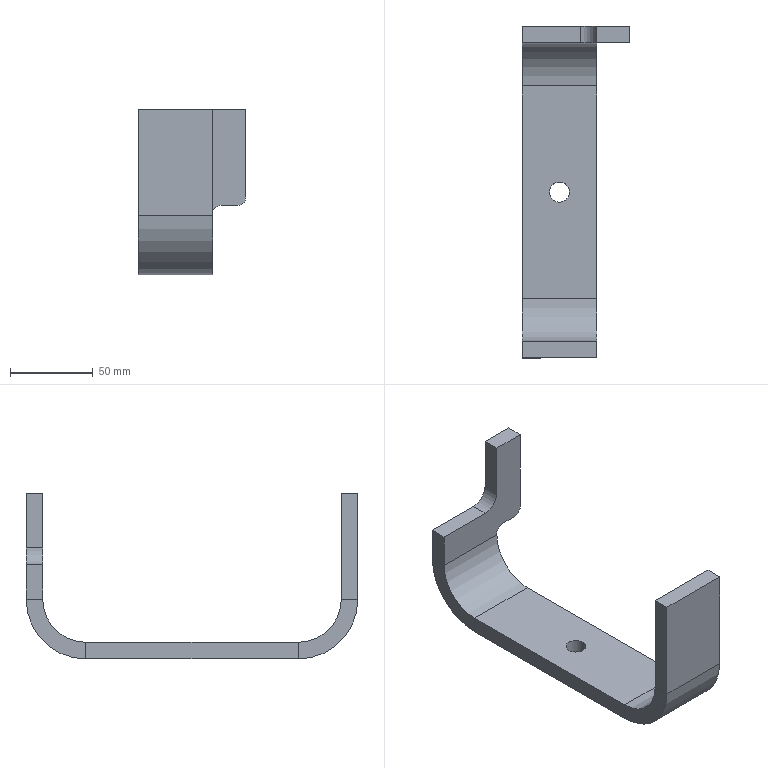Part | SolidWorks | features Cut 1, FlatPattern 1, SM3dBend 1, SMBaseFlange 1, SheetMetal 1 | 1 solid | 31 faces | box 65 x 200.003 x 99.994 mm | volume 150355 mm3 | plane 22 | cylinder 9 | commonest cylinder face diameters 10 x2 12 x2 52 x2 72 x2 20 x1
STEP:
#1=CARTESIAN_POINT('',(-38.456,6.751,0.));
#2=VERTEX_POINT('',#1);
#3=CARTESIAN_POINT('',(-26.456,6.751,0.));
#4=VERTEX_POINT('',#3);
#5=CARTESIAN_POINT('',(-32.456,6.751,0.));
#6=DIRECTION('',(0.,0.,1.));
#7=DIRECTION('',(1.,0.,0.));
#8=AXIS2_PLACEMENT_3D('',#5,#6,#7);
#9=CIRCLE('',#8,6.);
#10=EDGE_CURVE('',#2,#4,#9,.T.);
#11=ORIENTED_EDGE('',*,*,#10,.T.);
#12=CARTESIAN_POINT('',(-26.456,6.751,-10.));
#13=VERTEX_POINT('',#12);
#14=CARTESIAN_POINT('',(-26.456,6.751,89.994));
#15=DIRECTION('',(0.,0.,-1.));
#16=VECTOR('',#15,1000.);
#17=LINE('',#14,#16);
#18=EDGE_CURVE('',#4,#13,#17,.T.);
#19=ORIENTED_EDGE('',*,*,#18,.T.);
#20=CARTESIAN_POINT('',(-38.456,6.751,-10.));
#21=VERTEX_POINT('',#20);
#22=CARTESIAN_POINT('',(-32.456,6.751,-10.));
#23=DIRECTION('',(0.,0.,-1.));
#24=DIRECTION('',(-1.,0.,0.));
#25=AXIS2_PLACEMENT_3D('',#22,#23,#24);
#26=CIRCLE('',#25,6.);
#27=EDGE_CURVE('',#13,#21,#26,.T.);
#28=ORIENTED_EDGE('',*,*,#27,.T.);
#29=CARTESIAN_POINT('',(-38.456,6.751,89.994));
#30=DIRECTION('',(0.,0.,-1.));
#31=VECTOR('',#30,1000.);
#32=LINE('',#29,#31);
#33=EDGE_CURVE('',#2,#21,#32,.T.);
#34=ORIENTED_EDGE('',*,*,#33,.F.);
#35=EDGE_LOOP('',(#11,#19,#28,#34));
#36=FACE_OUTER_BOUND('',#35,.T.);
#37=CARTESIAN_POINT('',(-32.456,6.751,89.994));
#38=DIRECTION('',(0.,0.,-1.));
#39=DIRECTION('',(-1.,0.,0.));
#40=AXIS2_PLACEMENT_3D('',#37,#38,#39);
#41=CYLINDRICAL_SURFACE('',#40,6.);
#42=ADVANCED_FACE('',(#36),#41,.F.);
#43=CARTESIAN_POINT('',(-54.956,70.753,-10.));
#44=VERTEX_POINT('',#43);
#45=CARTESIAN_POINT('',(-54.956,-57.25,-10.));
#46=VERTEX_POINT('',#45);
#47=CARTESIAN_POINT('',(-54.956,-169.939,-10.));
#48=DIRECTION('',(0.,-1.,0.));
#49=VECTOR('',#48,1000.);
#50=LINE('',#47,#49);
#51=EDGE_CURVE('',#44,#46,#50,.T.);
#52=ORIENTED_EDGE('',*,*,#51,.T.);
#53=CARTESIAN_POINT('',(-54.956,-57.25,0.));
#54=VERTEX_POINT('',#53);
#55=CARTESIAN_POINT('',(-54.956,-57.25,-10.));
#56=DIRECTION('',(0.,0.,1.));
#57=VECTOR('',#56,1000.);
#58=LINE('',#55,#57);
#59=EDGE_CURVE('',#46,#54,#58,.T.);
#60=ORIENTED_EDGE('',*,*,#59,.T.);
#61=CARTESIAN_POINT('',(-54.956,70.753,0.));
#62=VERTEX_POINT('',#61);
#63=CARTESIAN_POINT('',(-54.956,-169.939,0.));
#64=DIRECTION('',(0.,-1.,0.));
#65=VECTOR('',#64,1000.);
#66=LINE('',#63,#65);
#67=EDGE_CURVE('',#62,#54,#66,.T.);
#68=ORIENTED_EDGE('',*,*,#67,.F.);
#69=CARTESIAN_POINT('',(-54.956,70.753,-10.));
#70=DIRECTION('',(0.,0.,1.));
#71=VECTOR('',#70,1000.);
#72=LINE('',#69,#71);
#73=EDGE_CURVE('',#44,#62,#72,.T.);
#74=ORIENTED_EDGE('',*,*,#73,.F.);
#75=EDGE_LOOP('',(#52,#60,#68,#74));
#76=FACE_OUTER_BOUND('',#75,.T.);
#77=CARTESIAN_POINT('',(-54.956,-169.939,-10.));
#78=DIRECTION('',(-1.,0.,0.));
#79=DIRECTION('',(0.,-1.,0.));
#80=AXIS2_PLACEMENT_3D('',#77,#78,#79);
#81=PLANE('',#80);
#82=ADVANCED_FACE('',(#76),#81,.T.);
#83=CARTESIAN_POINT('',(-9.956,-57.25,0.));
#84=VERTEX_POINT('',#83);
#85=CARTESIAN_POINT('',(-9.956,70.753,0.));
#86=VERTEX_POINT('',#85);
#87=CARTESIAN_POINT('',(-9.956,120.441,0.));
#88=DIRECTION('',(0.,1.,0.));
#89=VECTOR('',#88,1000.);
#90=LINE('',#87,#89);
#91=EDGE_CURVE('',#84,#86,#90,.T.);
#92=ORIENTED_EDGE('',*,*,#91,.F.);
#93=CARTESIAN_POINT('',(-9.956,-57.25,-10.));
#94=VERTEX_POINT('',#93);
#95=CARTESIAN_POINT('',(-9.956,-57.25,-10.));
#96=DIRECTION('',(0.,0.,-1.));
#97=VECTOR('',#96,1000.);
#98=LINE('',#95,#97);
#99=EDGE_CURVE('',#84,#94,#98,.T.);
#100=ORIENTED_EDGE('',*,*,#99,.T.);
#101=CARTESIAN_POINT('',(-9.956,70.753,-10.));
#102=VERTEX_POINT('',#101);
#103=CARTESIAN_POINT('',(-9.956,120.441,-10.));
#104=DIRECTION('',(0.,1.,0.));
#105=VECTOR('',#104,1000.);
#106=LINE('',#103,#105);
#107=EDGE_CURVE('',#94,#102,#106,.T.);
#108=ORIENTED_EDGE('',*,*,#107,.T.);
#109=CARTESIAN_POINT('',(-9.956,70.753,-10.));
#110=DIRECTION('',(0.,0.,-1.));
#111=VECTOR('',#110,1000.);
#112=LINE('',#109,#111);
#113=EDGE_CURVE('',#86,#102,#112,.T.);
#114=ORIENTED_EDGE('',*,*,#113,.F.);
#115=EDGE_LOOP('',(#92,#100,#108,#114));
#116=FACE_OUTER_BOUND('',#115,.T.);
#117=CARTESIAN_POINT('',(-9.956,120.441,-10.));
#118=DIRECTION('',(1.,0.,0.));
#119=DIRECTION('',(0.,0.,-1.));
#120=AXIS2_PLACEMENT_3D('',#117,#118,#119);
#121=PLANE('',#120);
#122=ADVANCED_FACE('',(#116),#121,.T.);
#123=ORIENTED_EDGE('',*,*,#10,.F.);
#124=CARTESIAN_POINT('',(-32.456,6.751,0.));
#125=DIRECTION('',(0.,0.,1.));
#126=DIRECTION('',(1.,0.,0.));
#127=AXIS2_PLACEMENT_3D('',#124,#125,#126);
#128=CIRCLE('',#127,6.);
#129=EDGE_CURVE('',#4,#2,#128,.T.);
#130=ORIENTED_EDGE('',*,*,#129,.F.);
#131=EDGE_LOOP('',(#123,#130));
#132=FACE_BOUND('',#131,.T.);
#133=ORIENTED_EDGE('',*,*,#67,.T.);
#134=CARTESIAN_POINT('',(-19.956,-57.25,0.));
#135=DIRECTION('',(1.,0.,0.));
#136=VECTOR('',#135,1000.);
#137=LINE('',#134,#136);
#138=EDGE_CURVE('',#54,#84,#137,.T.);
#139=ORIENTED_EDGE('',*,*,#138,.T.);
#140=ORIENTED_EDGE('',*,*,#91,.T.);
#141=CARTESIAN_POINT('',(-19.956,70.753,0.));
#142=DIRECTION('',(1.,0.,0.));
#143=VECTOR('',#142,1000.);
#144=LINE('',#141,#143);
#145=EDGE_CURVE('',#62,#86,#144,.T.);
#146=ORIENTED_EDGE('',*,*,#145,.F.);
#147=EDGE_LOOP('',(#133,#139,#140,#146));
#148=FACE_OUTER_BOUND('',#147,.T.);
#149=CARTESIAN_POINT('',(-19.956,150.441,0.));
#150=DIRECTION('',(0.,0.,1.));
#151=DIRECTION('',(1.,0.,0.));
#152=AXIS2_PLACEMENT_3D('',#149,#150,#151);
#153=PLANE('',#152);
#154=ADVANCED_FACE('',(#132,#148),#153,.T.);
#155=CARTESIAN_POINT('',(-32.456,6.751,-10.));
#156=DIRECTION('',(0.,0.,-1.));
#157=DIRECTION('',(-1.,0.,0.));
#158=AXIS2_PLACEMENT_3D('',#155,#156,#157);
#159=CIRCLE('',#158,6.);
#160=EDGE_CURVE('',#21,#13,#159,.T.);
#161=ORIENTED_EDGE('',*,*,#160,.F.);
#162=ORIENTED_EDGE('',*,*,#27,.F.);
#163=EDGE_LOOP('',(#161,#162));
#164=FACE_BOUND('',#163,.T.);
#165=CARTESIAN_POINT('',(-19.956,-57.25,-10.));
#166=DIRECTION('',(1.,0.,0.));
#167=VECTOR('',#166,1000.);
#168=LINE('',#165,#167);
#169=EDGE_CURVE('',#46,#94,#168,.T.);
#170=ORIENTED_EDGE('',*,*,#169,.F.);
#171=ORIENTED_EDGE('',*,*,#51,.F.);
#172=CARTESIAN_POINT('',(-19.956,70.753,-10.));
#173=DIRECTION('',(1.,0.,0.));
#174=VECTOR('',#173,1000.);
#175=LINE('',#172,#174);
#176=EDGE_CURVE('',#44,#102,#175,.T.);
#177=ORIENTED_EDGE('',*,*,#176,.T.);
#178=ORIENTED_EDGE('',*,*,#107,.F.);
#179=EDGE_LOOP('',(#170,#171,#177,#178));
#180=FACE_OUTER_BOUND('',#179,.T.);
#181=CARTESIAN_POINT('',(-19.956,150.441,-10.));
#182=DIRECTION('',(0.,0.,1.));
#183=DIRECTION('',(1.,0.,0.));
#184=AXIS2_PLACEMENT_3D('',#181,#182,#183);
#185=PLANE('',#184);
#186=ADVANCED_FACE('',(#164,#180),#185,.F.);
#187=ORIENTED_EDGE('',*,*,#73,.T.);
#188=CARTESIAN_POINT('',(-54.956,96.753,26.));
#189=VERTEX_POINT('',#188);
#190=CARTESIAN_POINT('',(-54.956,70.753,26.));
#191=DIRECTION('',(1.,0.,0.));
#192=DIRECTION('',(0.,0.,-1.));
#193=AXIS2_PLACEMENT_3D('',#190,#191,#192);
#194=CIRCLE('',#193,26.);
#195=EDGE_CURVE('',#62,#189,#194,.T.);
#196=ORIENTED_EDGE('',*,*,#195,.T.);
#197=CARTESIAN_POINT('',(-54.956,106.753,26.));
#198=VERTEX_POINT('',#197);
#199=CARTESIAN_POINT('',(-54.956,106.753,26.));
#200=DIRECTION('',(0.,-1.,0.));
#201=VECTOR('',#200,1000.);
#202=LINE('',#199,#201);
#203=EDGE_CURVE('',#198,#189,#202,.T.);
#204=ORIENTED_EDGE('',*,*,#203,.F.);
#205=CARTESIAN_POINT('',(-54.956,70.753,26.));
#206=DIRECTION('',(1.,0.,0.));
#207=DIRECTION('',(0.,0.,1.));
#208=AXIS2_PLACEMENT_3D('',#205,#206,#207);
#209=CIRCLE('',#208,36.);
#210=EDGE_CURVE('',#44,#198,#209,.T.);
#211=ORIENTED_EDGE('',*,*,#210,.F.);
#212=EDGE_LOOP('',(#187,#196,#204,#211));
#213=FACE_OUTER_BOUND('',#212,.T.);
#214=CARTESIAN_POINT('',(-54.956,70.753,26.));
#215=DIRECTION('',(-1.,0.,0.));
#216=DIRECTION('',(0.,0.,1.));
#217=AXIS2_PLACEMENT_3D('',#214,#215,#216);
#218=PLANE('',#217);
#219=ADVANCED_FACE('',(#213),#218,.T.);
#220=CARTESIAN_POINT('',(-9.956,96.753,26.));
#221=VERTEX_POINT('',#220);
#222=CARTESIAN_POINT('',(-9.956,106.753,26.));
#223=VERTEX_POINT('',#222);
#224=CARTESIAN_POINT('',(-9.956,106.753,26.));
#225=DIRECTION('',(0.,1.,0.));
#226=VECTOR('',#225,1000.);
#227=LINE('',#224,#226);
#228=EDGE_CURVE('',#221,#223,#227,.T.);
#229=ORIENTED_EDGE('',*,*,#228,.F.);
#230=CARTESIAN_POINT('',(-9.956,70.753,26.));
#231=DIRECTION('',(-1.,0.,0.));
#232=DIRECTION('',(0.,0.,-1.));
#233=AXIS2_PLACEMENT_3D('',#230,#231,#232);
#234=CIRCLE('',#233,26.);
#235=EDGE_CURVE('',#221,#86,#234,.T.);
#236=ORIENTED_EDGE('',*,*,#235,.T.);
#237=ORIENTED_EDGE('',*,*,#113,.T.);
#238=CARTESIAN_POINT('',(-9.956,70.753,26.));
#239=DIRECTION('',(-1.,0.,0.));
#240=DIRECTION('',(0.,0.,-1.));
#241=AXIS2_PLACEMENT_3D('',#238,#239,#240);
#242=CIRCLE('',#241,36.);
#243=EDGE_CURVE('',#223,#102,#242,.T.);
#244=ORIENTED_EDGE('',*,*,#243,.F.);
#245=EDGE_LOOP('',(#229,#236,#237,#244));
#246=FACE_OUTER_BOUND('',#245,.T.);
#247=CARTESIAN_POINT('',(-9.956,70.753,26.));
#248=DIRECTION('',(1.,0.,0.));
#249=DIRECTION('',(0.,0.,-1.));
#250=AXIS2_PLACEMENT_3D('',#247,#248,#249);
#251=PLANE('',#250);
#252=ADVANCED_FACE('',(#246),#251,.T.);
#253=ORIENTED_EDGE('',*,*,#243,.T.);
#254=ORIENTED_EDGE('',*,*,#176,.F.);
#255=ORIENTED_EDGE('',*,*,#210,.T.);
#256=CARTESIAN_POINT('',(-19.956,106.753,26.));
#257=DIRECTION('',(1.,0.,0.));
#258=VECTOR('',#257,1000.);
#259=LINE('',#256,#258);
#260=EDGE_CURVE('',#198,#223,#259,.T.);
#261=ORIENTED_EDGE('',*,*,#260,.T.);
#262=EDGE_LOOP('',(#253,#254,#255,#261));
#263=FACE_OUTER_BOUND('',#262,.T.);
#264=CARTESIAN_POINT('',(-99.51,70.753,26.));
#265=DIRECTION('',(1.,0.,0.));
#266=DIRECTION('',(0.,0.,-1.));
#267=AXIS2_PLACEMENT_3D('',#264,#265,#266);
#268=CYLINDRICAL_SURFACE('',#267,36.);
#269=ADVANCED_FACE('',(#263),#268,.T.);
#270=ORIENTED_EDGE('',*,*,#235,.F.);
#271=CARTESIAN_POINT('',(-19.956,96.753,26.));
#272=DIRECTION('',(1.,0.,0.));
#273=VECTOR('',#272,1000.);
#274=LINE('',#271,#273);
#275=EDGE_CURVE('',#189,#221,#274,.T.);
#276=ORIENTED_EDGE('',*,*,#275,.F.);
#277=ORIENTED_EDGE('',*,*,#195,.F.);
#278=ORIENTED_EDGE('',*,*,#145,.T.);
#279=EDGE_LOOP('',(#270,#276,#277,#278));
#280=FACE_OUTER_BOUND('',#279,.T.);
#281=CARTESIAN_POINT('',(-99.51,70.753,26.));
#282=DIRECTION('',(1.,0.,0.));
#283=DIRECTION('',(0.,0.,-1.));
#284=AXIS2_PLACEMENT_3D('',#281,#282,#283);
#285=CYLINDRICAL_SURFACE('',#284,26.);
#286=ADVANCED_FACE('',(#280),#285,.F.);
#287=CARTESIAN_POINT('',(-9.956,96.753,26.994));
#288=VERTEX_POINT('',#287);
#289=CARTESIAN_POINT('',(-4.956,96.753,31.994));
#290=VERTEX_POINT('',#289);
#291=CARTESIAN_POINT('',(-4.956,96.753,26.994));
#292=DIRECTION('',(0.,1.,0.));
#293=DIRECTION('',(1.,0.,0.));
#294=AXIS2_PLACEMENT_3D('',#291,#292,#293);
#295=CIRCLE('',#294,5.);
#296=EDGE_CURVE('',#288,#290,#295,.T.);
#297=ORIENTED_EDGE('',*,*,#296,.F.);
#298=CARTESIAN_POINT('',(-9.956,106.753,26.994));
#299=VERTEX_POINT('',#298);
#300=CARTESIAN_POINT('',(-9.956,106.753,26.994));
#301=DIRECTION('',(0.,-1.,0.));
#302=VECTOR('',#301,1000.);
#303=LINE('',#300,#302);
#304=EDGE_CURVE('',#299,#288,#303,.T.);
#305=ORIENTED_EDGE('',*,*,#304,.F.);
#306=CARTESIAN_POINT('',(-4.956,106.753,31.994));
#307=VERTEX_POINT('',#306);
#308=CARTESIAN_POINT('',(-4.956,106.753,26.994));
#309=DIRECTION('',(0.,1.,0.));
#310=DIRECTION('',(1.,0.,0.));
#311=AXIS2_PLACEMENT_3D('',#308,#309,#310);
#312=CIRCLE('',#311,5.);
#313=EDGE_CURVE('',#299,#307,#312,.T.);
#314=ORIENTED_EDGE('',*,*,#313,.T.);
#315=CARTESIAN_POINT('',(-4.956,106.753,31.994));
#316=DIRECTION('',(0.,-1.,0.));
#317=VECTOR('',#316,1000.);
#318=LINE('',#315,#317);
#319=EDGE_CURVE('',#307,#290,#318,.T.);
#320=ORIENTED_EDGE('',*,*,#319,.T.);
#321=EDGE_LOOP('',(#297,#305,#314,#320));
#322=FACE_OUTER_BOUND('',#321,.T.);
#323=CARTESIAN_POINT('',(-4.956,106.753,26.994));
#324=DIRECTION('',(0.,-1.,0.));
#325=DIRECTION('',(1.,0.,0.));
#326=AXIS2_PLACEMENT_3D('',#323,#324,#325);
#327=CYLINDRICAL_SURFACE('',#326,5.);
#328=ADVANCED_FACE('',(#322),#327,.F.);
#329=CARTESIAN_POINT('',(5.044,96.753,31.994));
#330=VERTEX_POINT('',#329);
#331=CARTESIAN_POINT('',(5.044,96.753,31.994));
#332=DIRECTION('',(1.,0.,0.));
#333=VECTOR('',#332,1000.);
#334=LINE('',#331,#333);
#335=EDGE_CURVE('',#290,#330,#334,.T.);
#336=ORIENTED_EDGE('',*,*,#335,.F.);
#337=ORIENTED_EDGE('',*,*,#319,.F.);
#338=CARTESIAN_POINT('',(5.044,106.753,31.994));
#339=VERTEX_POINT('',#338);
#340=CARTESIAN_POINT('',(5.044,106.753,31.994));
#341=DIRECTION('',(1.,0.,0.));
#342=VECTOR('',#341,1000.);
#343=LINE('',#340,#342);
#344=EDGE_CURVE('',#307,#339,#343,.T.);
#345=ORIENTED_EDGE('',*,*,#344,.T.);
#346=CARTESIAN_POINT('',(5.044,106.753,31.994));
#347=DIRECTION('',(0.,-1.,0.));
#348=VECTOR('',#347,1000.);
#349=LINE('',#346,#348);
#350=EDGE_CURVE('',#339,#330,#349,.T.);
#351=ORIENTED_EDGE('',*,*,#350,.T.);
#352=EDGE_LOOP('',(#336,#337,#345,#351));
#353=FACE_OUTER_BOUND('',#352,.T.);
#354=CARTESIAN_POINT('',(5.044,106.753,31.994));
#355=DIRECTION('',(0.,0.,-1.));
#356=DIRECTION('',(0.,1.,0.));
#357=AXIS2_PLACEMENT_3D('',#354,#355,#356);
#358=PLANE('',#357);
#359=ADVANCED_FACE('',(#353),#358,.T.);
#360=CARTESIAN_POINT('',(10.044,96.753,36.994));
#361=VERTEX_POINT('',#360);
#362=CARTESIAN_POINT('',(5.044,96.753,36.994));
#363=DIRECTION('',(0.,-1.,0.));
#364=DIRECTION('',(-1.,0.,0.));
#365=AXIS2_PLACEMENT_3D('',#362,#363,#364);
#366=CIRCLE('',#365,5.);
#367=EDGE_CURVE('',#330,#361,#366,.T.);
#368=ORIENTED_EDGE('',*,*,#367,.F.);
#369=ORIENTED_EDGE('',*,*,#350,.F.);
#370=CARTESIAN_POINT('',(10.044,106.753,36.994));
#371=VERTEX_POINT('',#370);
#372=CARTESIAN_POINT('',(5.044,106.753,36.994));
#373=DIRECTION('',(0.,-1.,0.));
#374=DIRECTION('',(-1.,0.,0.));
#375=AXIS2_PLACEMENT_3D('',#372,#373,#374);
#376=CIRCLE('',#375,5.);
#377=EDGE_CURVE('',#339,#371,#376,.T.);
#378=ORIENTED_EDGE('',*,*,#377,.T.);
#379=CARTESIAN_POINT('',(10.044,106.753,36.994));
#380=DIRECTION('',(0.,-1.,0.));
#381=VECTOR('',#380,1000.);
#382=LINE('',#379,#381);
#383=EDGE_CURVE('',#371,#361,#382,.T.);
#384=ORIENTED_EDGE('',*,*,#383,.T.);
#385=EDGE_LOOP('',(#368,#369,#378,#384));
#386=FACE_OUTER_BOUND('',#385,.T.);
#387=CARTESIAN_POINT('',(5.044,106.753,36.994));
#388=DIRECTION('',(0.,-1.,0.));
#389=DIRECTION('',(1.,0.,0.));
#390=AXIS2_PLACEMENT_3D('',#387,#388,#389);
#391=CYLINDRICAL_SURFACE('',#390,5.);
#392=ADVANCED_FACE('',(#386),#391,.T.);
#393=CARTESIAN_POINT('',(10.044,96.753,89.994));
#394=VERTEX_POINT('',#393);
#395=CARTESIAN_POINT('',(10.044,96.753,89.994));
#396=DIRECTION('',(0.,0.,1.));
#397=VECTOR('',#396,1000.);
#398=LINE('',#395,#397);
#399=EDGE_CURVE('',#361,#394,#398,.T.);
#400=ORIENTED_EDGE('',*,*,#399,.F.);
#401=ORIENTED_EDGE('',*,*,#383,.F.);
#402=CARTESIAN_POINT('',(10.044,106.753,89.994));
#403=VERTEX_POINT('',#402);
#404=CARTESIAN_POINT('',(10.044,106.753,89.994));
#405=DIRECTION('',(0.,0.,1.));
#406=VECTOR('',#405,1000.);
#407=LINE('',#404,#406);
#408=EDGE_CURVE('',#371,#403,#407,.T.);
#409=ORIENTED_EDGE('',*,*,#408,.T.);
#410=CARTESIAN_POINT('',(10.044,106.753,89.994));
#411=DIRECTION('',(0.,-1.,0.));
#412=VECTOR('',#411,1000.);
#413=LINE('',#410,#412);
#414=EDGE_CURVE('',#403,#394,#413,.T.);
#415=ORIENTED_EDGE('',*,*,#414,.T.);
#416=EDGE_LOOP('',(#400,#401,#409,#415));
#417=FACE_OUTER_BOUND('',#416,.T.);
#418=CARTESIAN_POINT('',(10.044,106.753,89.994));
#419=DIRECTION('',(1.,0.,0.));
#420=DIRECTION('',(0.,0.,1.));
#421=AXIS2_PLACEMENT_3D('',#418,#419,#420);
#422=PLANE('',#421);
#423=ADVANCED_FACE('',(#417),#422,.T.);
#424=CARTESIAN_POINT('',(-9.956,96.753,89.994));
#425=VERTEX_POINT('',#424);
#426=CARTESIAN_POINT('',(-9.956,96.753,89.994));
#427=DIRECTION('',(-1.,0.,0.));
#428=VECTOR('',#427,1000.);
#429=LINE('',#426,#428);
#430=EDGE_CURVE('',#394,#425,#429,.T.);
#431=ORIENTED_EDGE('',*,*,#430,.F.);
#432=ORIENTED_EDGE('',*,*,#414,.F.);
#433=CARTESIAN_POINT('',(-9.956,106.753,89.994));
#434=VERTEX_POINT('',#433);
#435=CARTESIAN_POINT('',(-9.956,106.753,89.994));
#436=DIRECTION('',(-1.,0.,0.));
#437=VECTOR('',#436,1000.);
#438=LINE('',#435,#437);
#439=EDGE_CURVE('',#403,#434,#438,.T.);
#440=ORIENTED_EDGE('',*,*,#439,.T.);
#441=CARTESIAN_POINT('',(-9.956,106.753,89.994));
#442=DIRECTION('',(0.,-1.,0.));
#443=VECTOR('',#442,1000.);
#444=LINE('',#441,#443);
#445=EDGE_CURVE('',#434,#425,#444,.T.);
#446=ORIENTED_EDGE('',*,*,#445,.T.);
#447=EDGE_LOOP('',(#431,#432,#440,#446));
#448=FACE_OUTER_BOUND('',#447,.T.);
#449=CARTESIAN_POINT('',(-9.956,106.753,89.994));
#450=DIRECTION('',(0.,0.,1.));
#451=DIRECTION('',(0.,-1.,0.));
#452=AXIS2_PLACEMENT_3D('',#449,#450,#451);
#453=PLANE('',#452);
#454=ADVANCED_FACE('',(#448),#453,.T.);
#455=CARTESIAN_POINT('',(-9.956,96.753,56.994));
#456=VERTEX_POINT('',#455);
#457=CARTESIAN_POINT('',(-9.956,96.753,56.994));
#458=DIRECTION('',(0.,0.,-1.));
#459=VECTOR('',#458,1000.);
#460=LINE('',#457,#459);
#461=EDGE_CURVE('',#425,#456,#460,.T.);
#462=ORIENTED_EDGE('',*,*,#461,.F.);
#463=ORIENTED_EDGE('',*,*,#445,.F.);
#464=CARTESIAN_POINT('',(-9.956,106.753,56.994));
#465=VERTEX_POINT('',#464);
#466=CARTESIAN_POINT('',(-9.956,106.753,56.994));
#467=DIRECTION('',(0.,0.,-1.));
#468=VECTOR('',#467,1000.);
#469=LINE('',#466,#468);
#470=EDGE_CURVE('',#434,#465,#469,.T.);
#471=ORIENTED_EDGE('',*,*,#470,.T.);
#472=CARTESIAN_POINT('',(-9.956,106.753,56.994));
#473=DIRECTION('',(0.,-1.,0.));
#474=VECTOR('',#473,1000.);
#475=LINE('',#472,#474);
#476=EDGE_CURVE('',#465,#456,#475,.T.);
#477=ORIENTED_EDGE('',*,*,#476,.T.);
#478=EDGE_LOOP('',(#462,#463,#471,#477));
#479=FACE_OUTER_BOUND('',#478,.T.);
#480=CARTESIAN_POINT('',(-9.956,106.753,56.994));
#481=DIRECTION('',(-1.,0.,0.));
#482=DIRECTION('',(0.,-1.,0.));
#483=AXIS2_PLACEMENT_3D('',#480,#481,#482);
#484=PLANE('',#483);
#485=ADVANCED_FACE('',(#479),#484,.T.);
#486=CARTESIAN_POINT('',(-19.956,96.753,46.994));
#487=VERTEX_POINT('',#486);
#488=CARTESIAN_POINT('',(-19.956,96.753,56.994));
#489=DIRECTION('',(0.,1.,0.));
#490=DIRECTION('',(1.,0.,0.));
#491=AXIS2_PLACEMENT_3D('',#488,#489,#490);
#492=CIRCLE('',#491,10.);
#493=EDGE_CURVE('',#456,#487,#492,.T.);
#494=ORIENTED_EDGE('',*,*,#493,.F.);
#495=ORIENTED_EDGE('',*,*,#476,.F.);
#496=CARTESIAN_POINT('',(-19.956,106.753,46.994));
#497=VERTEX_POINT('',#496);
#498=CARTESIAN_POINT('',(-19.956,106.753,56.994));
#499=DIRECTION('',(0.,1.,0.));
#500=DIRECTION('',(1.,0.,0.));
#501=AXIS2_PLACEMENT_3D('',#498,#499,#500);
#502=CIRCLE('',#501,10.);
#503=EDGE_CURVE('',#465,#497,#502,.T.);
#504=ORIENTED_EDGE('',*,*,#503,.T.);
#505=CARTESIAN_POINT('',(-19.956,106.753,46.994));
#506=DIRECTION('',(0.,-1.,0.));
#507=VECTOR('',#506,1000.);
#508=LINE('',#505,#507);
#509=EDGE_CURVE('',#497,#487,#508,.T.);
#510=ORIENTED_EDGE('',*,*,#509,.T.);
#511=EDGE_LOOP('',(#494,#495,#504,#510));
#512=FACE_OUTER_BOUND('',#511,.T.);
#513=CARTESIAN_POINT('',(-19.956,106.753,56.994));
#514=DIRECTION('',(0.,-1.,0.));
#515=DIRECTION('',(1.,0.,0.));
#516=AXIS2_PLACEMENT_3D('',#513,#514,#515);
#517=CYLINDRICAL_SURFACE('',#516,10.);
#518=ADVANCED_FACE('',(#512),#517,.F.);
#519=CARTESIAN_POINT('',(-54.956,96.753,46.994));
#520=VERTEX_POINT('',#519);
#521=CARTESIAN_POINT('',(-54.956,96.753,46.994));
#522=DIRECTION('',(-1.,0.,0.));
#523=VECTOR('',#522,1000.);
#524=LINE('',#521,#523);
#525=EDGE_CURVE('',#487,#520,#524,.T.);
#526=ORIENTED_EDGE('',*,*,#525,.F.);
#527=ORIENTED_EDGE('',*,*,#509,.F.);
#528=CARTESIAN_POINT('',(-54.956,106.753,46.994));
#529=VERTEX_POINT('',#528);
#530=CARTESIAN_POINT('',(-54.956,106.753,46.994));
#531=DIRECTION('',(-1.,0.,0.));
#532=VECTOR('',#531,1000.);
#533=LINE('',#530,#532);
#534=EDGE_CURVE('',#497,#529,#533,.T.);
#535=ORIENTED_EDGE('',*,*,#534,.T.);
#536=CARTESIAN_POINT('',(-54.956,106.753,46.994));
#537=DIRECTION('',(0.,-1.,0.));
#538=VECTOR('',#537,1000.);
#539=LINE('',#536,#538);
#540=EDGE_CURVE('',#529,#520,#539,.T.);
#541=ORIENTED_EDGE('',*,*,#540,.T.);
#542=EDGE_LOOP('',(#526,#527,#535,#541));
#543=FACE_OUTER_BOUND('',#542,.T.);
#544=CARTESIAN_POINT('',(-54.956,106.753,46.994));
#545=DIRECTION('',(0.,0.,1.));
#546=DIRECTION('',(0.,-1.,0.));
#547=AXIS2_PLACEMENT_3D('',#544,#545,#546);
#548=PLANE('',#547);
#549=ADVANCED_FACE('',(#543),#548,.T.);
#550=ORIENTED_EDGE('',*,*,#260,.F.);
#551=CARTESIAN_POINT('',(-54.956,106.753,-263.386));
#552=DIRECTION('',(0.,0.,-1.));
#553=VECTOR('',#552,1000.);
#554=LINE('',#551,#553);
#555=EDGE_CURVE('',#529,#198,#554,.T.);
#556=ORIENTED_EDGE('',*,*,#555,.F.);
#557=ORIENTED_EDGE('',*,*,#534,.F.);
#558=ORIENTED_EDGE('',*,*,#503,.F.);
#559=ORIENTED_EDGE('',*,*,#470,.F.);
#560=ORIENTED_EDGE('',*,*,#439,.F.);
#561=ORIENTED_EDGE('',*,*,#408,.F.);
#562=ORIENTED_EDGE('',*,*,#377,.F.);
#563=ORIENTED_EDGE('',*,*,#344,.F.);
#564=ORIENTED_EDGE('',*,*,#313,.F.);
#565=CARTESIAN_POINT('',(-9.956,106.753,26.994));
#566=DIRECTION('',(0.,0.,1.));
#567=VECTOR('',#566,1000.);
#568=LINE('',#565,#567);
#569=EDGE_CURVE('',#223,#299,#568,.T.);
#570=ORIENTED_EDGE('',*,*,#569,.F.);
#571=EDGE_LOOP('',(#550,#556,#557,#558,#559,#560,#561,#562,#563,#564,#570));
#572=FACE_OUTER_BOUND('',#571,.T.);
#573=CARTESIAN_POINT('',(-19.956,106.753,56.994));
#574=DIRECTION('',(0.,-1.,0.));
#575=DIRECTION('',(1.,0.,0.));
#576=AXIS2_PLACEMENT_3D('',#573,#574,#575);
#577=PLANE('',#576);
#578=ADVANCED_FACE('',(#572),#577,.F.);
#579=ORIENTED_EDGE('',*,*,#555,.T.);
#580=ORIENTED_EDGE('',*,*,#203,.T.);
#581=CARTESIAN_POINT('',(-54.956,96.753,-263.386));
#582=DIRECTION('',(0.,0.,-1.));
#583=VECTOR('',#582,1000.);
#584=LINE('',#581,#583);
#585=EDGE_CURVE('',#520,#189,#584,.T.);
#586=ORIENTED_EDGE('',*,*,#585,.F.);
#587=ORIENTED_EDGE('',*,*,#540,.F.);
#588=EDGE_LOOP('',(#579,#580,#586,#587));
#589=FACE_OUTER_BOUND('',#588,.T.);
#590=CARTESIAN_POINT('',(-54.956,106.753,-263.386));
#591=DIRECTION('',(-1.,0.,0.));
#592=DIRECTION('',(0.,0.,-1.));
#593=AXIS2_PLACEMENT_3D('',#590,#591,#592);
#594=PLANE('',#593);
#595=ADVANCED_FACE('',(#589),#594,.T.);
#596=ORIENTED_EDGE('',*,*,#585,.T.);
#597=ORIENTED_EDGE('',*,*,#275,.T.);
#598=CARTESIAN_POINT('',(-9.956,96.753,26.994));
#599=DIRECTION('',(0.,0.,1.));
#600=VECTOR('',#599,1000.);
#601=LINE('',#598,#600);
#602=EDGE_CURVE('',#221,#288,#601,.T.);
#603=ORIENTED_EDGE('',*,*,#602,.T.);
#604=ORIENTED_EDGE('',*,*,#296,.T.);
#605=ORIENTED_EDGE('',*,*,#335,.T.);
#606=ORIENTED_EDGE('',*,*,#367,.T.);
#607=ORIENTED_EDGE('',*,*,#399,.T.);
#608=ORIENTED_EDGE('',*,*,#430,.T.);
#609=ORIENTED_EDGE('',*,*,#461,.T.);
#610=ORIENTED_EDGE('',*,*,#493,.T.);
#611=ORIENTED_EDGE('',*,*,#525,.T.);
#612=EDGE_LOOP('',(#596,#597,#603,#604,#605,#606,#607,#608,#609,#610,#611));
#613=FACE_OUTER_BOUND('',#612,.T.);
#614=CARTESIAN_POINT('',(-19.956,96.753,56.994));
#615=DIRECTION('',(0.,-1.,0.));
#616=DIRECTION('',(1.,0.,0.));
#617=AXIS2_PLACEMENT_3D('',#614,#615,#616);
#618=PLANE('',#617);
#619=ADVANCED_FACE('',(#613),#618,.T.);
#620=ORIENTED_EDGE('',*,*,#602,.F.);
#621=ORIENTED_EDGE('',*,*,#228,.T.);
#622=ORIENTED_EDGE('',*,*,#569,.T.);
#623=ORIENTED_EDGE('',*,*,#304,.T.);
#624=EDGE_LOOP('',(#620,#621,#622,#623));
#625=FACE_OUTER_BOUND('',#624,.T.);
#626=CARTESIAN_POINT('',(-9.956,106.753,26.994));
#627=DIRECTION('',(1.,0.,0.));
#628=DIRECTION('',(0.,1.,0.));
#629=AXIS2_PLACEMENT_3D('',#626,#627,#628);
#630=PLANE('',#629);
#631=ADVANCED_FACE('',(#625),#630,.T.);
#632=CARTESIAN_POINT('',(-54.956,-93.25,26.));
#633=VERTEX_POINT('',#632);
#634=CARTESIAN_POINT('',(-54.956,-83.25,26.));
#635=VERTEX_POINT('',#634);
#636=CARTESIAN_POINT('',(-54.956,-93.25,26.));
#637=DIRECTION('',(0.,1.,0.));
#638=VECTOR('',#637,1000.);
#639=LINE('',#636,#638);
#640=EDGE_CURVE('',#633,#635,#639,.T.);
#641=ORIENTED_EDGE('',*,*,#640,.T.);
#642=CARTESIAN_POINT('',(-54.956,-57.25,26.));
#643=DIRECTION('',(1.,0.,0.));
#644=DIRECTION('',(0.,-1.,0.));
#645=AXIS2_PLACEMENT_3D('',#642,#643,#644);
#646=CIRCLE('',#645,26.);
#647=EDGE_CURVE('',#635,#54,#646,.T.);
#648=ORIENTED_EDGE('',*,*,#647,.T.);
#649=ORIENTED_EDGE('',*,*,#59,.F.);
#650=CARTESIAN_POINT('',(-54.956,-57.25,26.));
#651=DIRECTION('',(1.,0.,0.));
#652=DIRECTION('',(0.,0.,1.));
#653=AXIS2_PLACEMENT_3D('',#650,#651,#652);
#654=CIRCLE('',#653,36.);
#655=EDGE_CURVE('',#633,#46,#654,.T.);
#656=ORIENTED_EDGE('',*,*,#655,.F.);
#657=EDGE_LOOP('',(#641,#648,#649,#656));
#658=FACE_OUTER_BOUND('',#657,.T.);
#659=CARTESIAN_POINT('',(-54.956,-57.25,26.));
#660=DIRECTION('',(-1.,0.,0.));
#661=DIRECTION('',(0.,0.,1.));
#662=AXIS2_PLACEMENT_3D('',#659,#660,#661);
#663=PLANE('',#662);
#664=ADVANCED_FACE('',(#658),#663,.T.);
#665=ORIENTED_EDGE('',*,*,#99,.F.);
#666=CARTESIAN_POINT('',(-9.956,-83.25,26.));
#667=VERTEX_POINT('',#666);
#668=CARTESIAN_POINT('',(-9.956,-57.25,26.));
#669=DIRECTION('',(-1.,0.,0.));
#670=DIRECTION('',(0.,-1.,0.));
#671=AXIS2_PLACEMENT_3D('',#668,#669,#670);
#672=CIRCLE('',#671,26.);
#673=EDGE_CURVE('',#84,#667,#672,.T.);
#674=ORIENTED_EDGE('',*,*,#673,.T.);
#675=CARTESIAN_POINT('',(-9.956,-93.25,26.));
#676=VERTEX_POINT('',#675);
#677=CARTESIAN_POINT('',(-9.956,-93.25,26.));
#678=DIRECTION('',(0.,-1.,0.));
#679=VECTOR('',#678,1000.);
#680=LINE('',#677,#679);
#681=EDGE_CURVE('',#667,#676,#680,.T.);
#682=ORIENTED_EDGE('',*,*,#681,.T.);
#683=CARTESIAN_POINT('',(-9.956,-57.25,26.));
#684=DIRECTION('',(-1.,0.,0.));
#685=DIRECTION('',(0.,1.,0.));
#686=AXIS2_PLACEMENT_3D('',#683,#684,#685);
#687=CIRCLE('',#686,36.);
#688=EDGE_CURVE('',#94,#676,#687,.T.);
#689=ORIENTED_EDGE('',*,*,#688,.F.);
#690=EDGE_LOOP('',(#665,#674,#682,#689));
#691=FACE_OUTER_BOUND('',#690,.T.);
#692=CARTESIAN_POINT('',(-9.956,-57.25,26.));
#693=DIRECTION('',(1.,0.,0.));
#694=DIRECTION('',(0.,1.,0.));
#695=AXIS2_PLACEMENT_3D('',#692,#693,#694);
#696=PLANE('',#695);
#697=ADVANCED_FACE('',(#691),#696,.T.);
#698=ORIENTED_EDGE('',*,*,#688,.T.);
#699=CARTESIAN_POINT('',(-19.956,-93.25,26.));
#700=DIRECTION('',(1.,0.,0.));
#701=VECTOR('',#700,1000.);
#702=LINE('',#699,#701);
#703=EDGE_CURVE('',#633,#676,#702,.T.);
#704=ORIENTED_EDGE('',*,*,#703,.F.);
#705=ORIENTED_EDGE('',*,*,#655,.T.);
#706=ORIENTED_EDGE('',*,*,#169,.T.);
#707=EDGE_LOOP('',(#698,#704,#705,#706));
#708=FACE_OUTER_BOUND('',#707,.T.);
#709=CARTESIAN_POINT('',(34.597,-57.25,26.));
#710=DIRECTION('',(-1.,0.,0.));
#711=DIRECTION('',(0.,-1.,0.));
#712=AXIS2_PLACEMENT_3D('',#709,#710,#711);
#713=CYLINDRICAL_SURFACE('',#712,36.);
#714=ADVANCED_FACE('',(#708),#713,.T.);
#715=ORIENTED_EDGE('',*,*,#673,.F.);
#716=ORIENTED_EDGE('',*,*,#138,.F.);
#717=ORIENTED_EDGE('',*,*,#647,.F.);
#718=CARTESIAN_POINT('',(-19.956,-83.25,26.));
#719=DIRECTION('',(1.,0.,0.));
#720=VECTOR('',#719,1000.);
#721=LINE('',#718,#720);
#722=EDGE_CURVE('',#635,#667,#721,.T.);
#723=ORIENTED_EDGE('',*,*,#722,.T.);
#724=EDGE_LOOP('',(#715,#716,#717,#723));
#725=FACE_OUTER_BOUND('',#724,.T.);
#726=CARTESIAN_POINT('',(34.597,-57.25,26.));
#727=DIRECTION('',(-1.,0.,0.));
#728=DIRECTION('',(0.,-1.,0.));
#729=AXIS2_PLACEMENT_3D('',#726,#727,#728);
#730=CYLINDRICAL_SURFACE('',#729,26.);
#731=ADVANCED_FACE('',(#725),#730,.F.);
#732=CARTESIAN_POINT('',(-54.956,-83.25,89.994));
#733=VERTEX_POINT('',#732);
#734=CARTESIAN_POINT('',(-9.956,-83.25,89.994));
#735=VERTEX_POINT('',#734);
#736=CARTESIAN_POINT('',(-9.956,-83.25,89.994));
#737=DIRECTION('',(1.,0.,0.));
#738=VECTOR('',#737,1000.);
#739=LINE('',#736,#738);
#740=EDGE_CURVE('',#733,#735,#739,.T.);
#741=ORIENTED_EDGE('',*,*,#740,.F.);
#742=CARTESIAN_POINT('',(-54.956,-93.25,89.994));
#743=VERTEX_POINT('',#742);
#744=CARTESIAN_POINT('',(-54.956,-93.25,89.994));
#745=DIRECTION('',(0.,1.,0.));
#746=VECTOR('',#745,1000.);
#747=LINE('',#744,#746);
#748=EDGE_CURVE('',#743,#733,#747,.T.);
#749=ORIENTED_EDGE('',*,*,#748,.F.);
#750=CARTESIAN_POINT('',(-9.956,-93.25,89.994));
#751=VERTEX_POINT('',#750);
#752=CARTESIAN_POINT('',(-9.956,-93.25,89.994));
#753=DIRECTION('',(1.,0.,0.));
#754=VECTOR('',#753,1000.);
#755=LINE('',#752,#754);
#756=EDGE_CURVE('',#743,#751,#755,.T.);
#757=ORIENTED_EDGE('',*,*,#756,.T.);
#758=CARTESIAN_POINT('',(-9.956,-93.25,89.994));
#759=DIRECTION('',(0.,1.,0.));
#760=VECTOR('',#759,1000.);
#761=LINE('',#758,#760);
#762=EDGE_CURVE('',#751,#735,#761,.T.);
#763=ORIENTED_EDGE('',*,*,#762,.T.);
#764=EDGE_LOOP('',(#741,#749,#757,#763));
#765=FACE_OUTER_BOUND('',#764,.T.);
#766=CARTESIAN_POINT('',(-9.956,-93.25,89.994));
#767=DIRECTION('',(0.,0.,1.));
#768=DIRECTION('',(0.,-1.,0.));
#769=AXIS2_PLACEMENT_3D('',#766,#767,#768);
#770=PLANE('',#769);
#771=ADVANCED_FACE('',(#765),#770,.T.);
#772=CARTESIAN_POINT('',(-54.956,-93.25,89.994));
#773=DIRECTION('',(0.,0.,1.));
#774=VECTOR('',#773,1000.);
#775=LINE('',#772,#774);
#776=EDGE_CURVE('',#633,#743,#775,.T.);
#777=ORIENTED_EDGE('',*,*,#776,.F.);
#778=ORIENTED_EDGE('',*,*,#703,.T.);
#779=CARTESIAN_POINT('',(-9.956,-93.25,-200.386));
#780=DIRECTION('',(0.,0.,-1.));
#781=VECTOR('',#780,1000.);
#782=LINE('',#779,#781);
#783=EDGE_CURVE('',#751,#676,#782,.T.);
#784=ORIENTED_EDGE('',*,*,#783,.F.);
#785=ORIENTED_EDGE('',*,*,#756,.F.);
#786=EDGE_LOOP('',(#777,#778,#784,#785));
#787=FACE_OUTER_BOUND('',#786,.T.);
#788=CARTESIAN_POINT('',(-19.956,-93.25,-230.386));
#789=DIRECTION('',(0.,1.,0.));
#790=DIRECTION('',(1.,0.,0.));
#791=AXIS2_PLACEMENT_3D('',#788,#789,#790);
#792=PLANE('',#791);
#793=ADVANCED_FACE('',(#787),#792,.F.);
#794=ORIENTED_EDGE('',*,*,#681,.F.);
#795=CARTESIAN_POINT('',(-9.956,-83.25,-200.386));
#796=DIRECTION('',(0.,0.,-1.));
#797=VECTOR('',#796,1000.);
#798=LINE('',#795,#797);
#799=EDGE_CURVE('',#735,#667,#798,.T.);
#800=ORIENTED_EDGE('',*,*,#799,.F.);
#801=ORIENTED_EDGE('',*,*,#762,.F.);
#802=ORIENTED_EDGE('',*,*,#783,.T.);
#803=EDGE_LOOP('',(#794,#800,#801,#802));
#804=FACE_OUTER_BOUND('',#803,.T.);
#805=CARTESIAN_POINT('',(-9.956,-93.25,-200.386));
#806=DIRECTION('',(1.,0.,0.));
#807=DIRECTION('',(0.,-1.,0.));
#808=AXIS2_PLACEMENT_3D('',#805,#806,#807);
#809=PLANE('',#808);
#810=ADVANCED_FACE('',(#804),#809,.T.);
#811=ORIENTED_EDGE('',*,*,#722,.F.);
#812=CARTESIAN_POINT('',(-54.956,-83.25,89.994));
#813=DIRECTION('',(0.,0.,1.));
#814=VECTOR('',#813,1000.);
#815=LINE('',#812,#814);
#816=EDGE_CURVE('',#635,#733,#815,.T.);
#817=ORIENTED_EDGE('',*,*,#816,.T.);
#818=ORIENTED_EDGE('',*,*,#740,.T.);
#819=ORIENTED_EDGE('',*,*,#799,.T.);
#820=EDGE_LOOP('',(#811,#817,#818,#819));
#821=FACE_OUTER_BOUND('',#820,.T.);
#822=CARTESIAN_POINT('',(-19.956,-83.25,-230.386));
#823=DIRECTION('',(0.,1.,0.));
#824=DIRECTION('',(1.,0.,0.));
#825=AXIS2_PLACEMENT_3D('',#822,#823,#824);
#826=PLANE('',#825);
#827=ADVANCED_FACE('',(#821),#826,.T.);
#828=ORIENTED_EDGE('',*,*,#640,.F.);
#829=ORIENTED_EDGE('',*,*,#776,.T.);
#830=ORIENTED_EDGE('',*,*,#748,.T.);
#831=ORIENTED_EDGE('',*,*,#816,.F.);
#832=EDGE_LOOP('',(#828,#829,#830,#831));
#833=FACE_OUTER_BOUND('',#832,.T.);
#834=CARTESIAN_POINT('',(-54.956,-93.25,89.994));
#835=DIRECTION('',(-1.,0.,0.));
#836=DIRECTION('',(0.,0.,1.));
#837=AXIS2_PLACEMENT_3D('',#834,#835,#836);
#838=PLANE('',#837);
#839=ADVANCED_FACE('',(#833),#838,.T.);
#840=ORIENTED_EDGE('',*,*,#18,.F.);
#841=ORIENTED_EDGE('',*,*,#129,.T.);
#842=ORIENTED_EDGE('',*,*,#33,.T.);
#843=ORIENTED_EDGE('',*,*,#160,.T.);
#844=EDGE_LOOP('',(#840,#841,#842,#843));
#845=FACE_OUTER_BOUND('',#844,.T.);
#846=CARTESIAN_POINT('',(-32.456,6.751,89.994));
#847=DIRECTION('',(0.,0.,-1.));
#848=DIRECTION('',(-1.,0.,0.));
#849=AXIS2_PLACEMENT_3D('',#846,#847,#848);
#850=CYLINDRICAL_SURFACE('',#849,6.);
#851=ADVANCED_FACE('',(#845),#850,.F.);
#852=CLOSED_SHELL('',(#42,#82,#122,#154,#186,#219,#252,#269,#286,#328,#359,#392,#423,#454,#485,#518,#549,#578,#595,#619,#631,#664,#697,#714,#731,#771,#793,#810,#827,#839,#851));
#853=MANIFOLD_SOLID_BREP('',#852);
#854=CARTESIAN_POINT('',(0.,0.,0.));
#855=DIRECTION('',(0.,0.,1.));
#856=DIRECTION('',(1.,0.,0.));
#857=AXIS2_PLACEMENT_3D('',#854,#855,#856);
#858=(LENGTH_UNIT()NAMED_UNIT(*)SI_UNIT(.MILLI.,.METRE.));
#859=UNCERTAINTY_MEASURE_WITH_UNIT(LENGTH_MEASURE(0.00001),#858,'','');
#860=(NAMED_UNIT(*)PLANE_ANGLE_UNIT()SI_UNIT($,.RADIAN.));
#861=(NAMED_UNIT(*)SI_UNIT($,.STERADIAN.)SOLID_ANGLE_UNIT());
#862=(GEOMETRIC_REPRESENTATION_CONTEXT(3)GLOBAL_UNCERTAINTY_ASSIGNED_CONTEXT((#859))GLOBAL_UNIT_ASSIGNED_CONTEXT((#858,#860,#861))REPRESENTATION_CONTEXT('',''));
#863=ADVANCED_BREP_SHAPE_REPRESENTATION('',(#853,#857),#862);